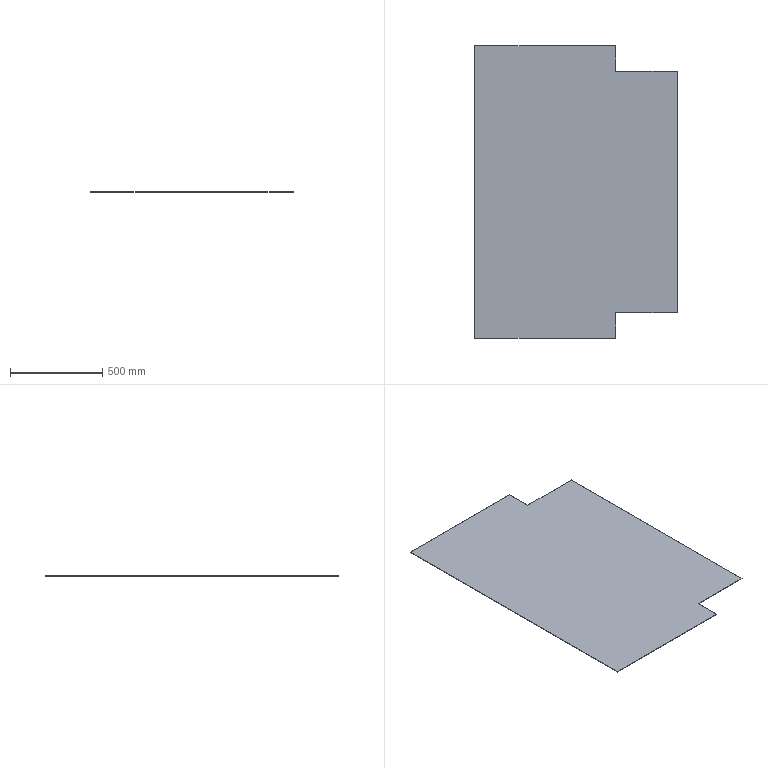Part | SolidWorks | 1 solid | 10 faces | box 1100 x 1590 x 2.5 mm | volume 4138000 mm3 | plane 10
STEP:
#1=CARTESIAN_POINT('',(-1620.,795.,0.));
#2=VERTEX_POINT('',#1);
#3=CARTESIAN_POINT('',(-1620.,-795.,0.));
#4=VERTEX_POINT('',#3);
#5=CARTESIAN_POINT('',(-1620.,795.,0.));
#6=DIRECTION('',(0.,-1.,0.));
#7=VECTOR('',#6,1000.);
#8=LINE('',#5,#7);
#9=EDGE_CURVE('',#2,#4,#8,.T.);
#10=ORIENTED_EDGE('',*,*,#9,.T.);
#11=CARTESIAN_POINT('',(-1620.,-795.,2.5));
#12=VERTEX_POINT('',#11);
#13=CARTESIAN_POINT('',(-1620.,-795.,2.5));
#14=DIRECTION('',(0.,0.,-1.));
#15=VECTOR('',#14,1000.);
#16=LINE('',#13,#15);
#17=EDGE_CURVE('',#12,#4,#16,.T.);
#18=ORIENTED_EDGE('',*,*,#17,.F.);
#19=CARTESIAN_POINT('',(-1620.,795.,2.5));
#20=VERTEX_POINT('',#19);
#21=CARTESIAN_POINT('',(-1620.,795.,2.5));
#22=DIRECTION('',(0.,-1.,0.));
#23=VECTOR('',#22,1000.);
#24=LINE('',#21,#23);
#25=EDGE_CURVE('',#20,#12,#24,.T.);
#26=ORIENTED_EDGE('',*,*,#25,.F.);
#27=CARTESIAN_POINT('',(-1620.,795.,2.5));
#28=DIRECTION('',(0.,0.,-1.));
#29=VECTOR('',#28,1000.);
#30=LINE('',#27,#29);
#31=EDGE_CURVE('',#20,#2,#30,.T.);
#32=ORIENTED_EDGE('',*,*,#31,.T.);
#33=EDGE_LOOP('',(#10,#18,#26,#32));
#34=FACE_OUTER_BOUND('',#33,.T.);
#35=CARTESIAN_POINT('',(-1620.,795.,2.5));
#36=DIRECTION('',(1.,0.,0.));
#37=DIRECTION('',(0.,1.,0.));
#38=AXIS2_PLACEMENT_3D('',#35,#36,#37);
#39=PLANE('',#38);
#40=ADVANCED_FACE('',(#34),#39,.F.);
#41=CARTESIAN_POINT('',(-855.,-795.,0.));
#42=VERTEX_POINT('',#41);
#43=CARTESIAN_POINT('',(-1620.,-795.,0.));
#44=DIRECTION('',(1.,0.,0.));
#45=VECTOR('',#44,1000.);
#46=LINE('',#43,#45);
#47=EDGE_CURVE('',#4,#42,#46,.T.);
#48=ORIENTED_EDGE('',*,*,#47,.T.);
#49=CARTESIAN_POINT('',(-855.,-795.,2.5));
#50=VERTEX_POINT('',#49);
#51=CARTESIAN_POINT('',(-855.,-795.,2.5));
#52=DIRECTION('',(0.,0.,-1.));
#53=VECTOR('',#52,1000.);
#54=LINE('',#51,#53);
#55=EDGE_CURVE('',#50,#42,#54,.T.);
#56=ORIENTED_EDGE('',*,*,#55,.F.);
#57=CARTESIAN_POINT('',(-1620.,-795.,2.5));
#58=DIRECTION('',(1.,0.,0.));
#59=VECTOR('',#58,1000.);
#60=LINE('',#57,#59);
#61=EDGE_CURVE('',#12,#50,#60,.T.);
#62=ORIENTED_EDGE('',*,*,#61,.F.);
#63=ORIENTED_EDGE('',*,*,#17,.T.);
#64=EDGE_LOOP('',(#48,#56,#62,#63));
#65=FACE_OUTER_BOUND('',#64,.T.);
#66=CARTESIAN_POINT('',(-1620.,-795.,2.5));
#67=DIRECTION('',(0.,1.,0.));
#68=DIRECTION('',(0.,0.,1.));
#69=AXIS2_PLACEMENT_3D('',#66,#67,#68);
#70=PLANE('',#69);
#71=ADVANCED_FACE('',(#65),#70,.F.);
#72=CARTESIAN_POINT('',(-855.,-655.,0.));
#73=VERTEX_POINT('',#72);
#74=CARTESIAN_POINT('',(-855.,-795.,0.));
#75=DIRECTION('',(0.,1.,0.));
#76=VECTOR('',#75,1000.);
#77=LINE('',#74,#76);
#78=EDGE_CURVE('',#42,#73,#77,.T.);
#79=ORIENTED_EDGE('',*,*,#78,.T.);
#80=CARTESIAN_POINT('',(-855.,-655.,2.5));
#81=VERTEX_POINT('',#80);
#82=CARTESIAN_POINT('',(-855.,-655.,2.5));
#83=DIRECTION('',(0.,0.,-1.));
#84=VECTOR('',#83,1000.);
#85=LINE('',#82,#84);
#86=EDGE_CURVE('',#81,#73,#85,.T.);
#87=ORIENTED_EDGE('',*,*,#86,.F.);
#88=CARTESIAN_POINT('',(-855.,-795.,2.5));
#89=DIRECTION('',(0.,1.,0.));
#90=VECTOR('',#89,1000.);
#91=LINE('',#88,#90);
#92=EDGE_CURVE('',#50,#81,#91,.T.);
#93=ORIENTED_EDGE('',*,*,#92,.F.);
#94=ORIENTED_EDGE('',*,*,#55,.T.);
#95=EDGE_LOOP('',(#79,#87,#93,#94));
#96=FACE_OUTER_BOUND('',#95,.T.);
#97=CARTESIAN_POINT('',(-855.,-795.,2.5));
#98=DIRECTION('',(-1.,0.,0.));
#99=DIRECTION('',(0.,0.,1.));
#100=AXIS2_PLACEMENT_3D('',#97,#98,#99);
#101=PLANE('',#100);
#102=ADVANCED_FACE('',(#96),#101,.F.);
#103=CARTESIAN_POINT('',(-520.,-655.,0.));
#104=VERTEX_POINT('',#103);
#105=CARTESIAN_POINT('',(-855.,-655.,0.));
#106=DIRECTION('',(1.,0.,0.));
#107=VECTOR('',#106,1000.);
#108=LINE('',#105,#107);
#109=EDGE_CURVE('',#73,#104,#108,.T.);
#110=ORIENTED_EDGE('',*,*,#109,.T.);
#111=CARTESIAN_POINT('',(-520.,-655.,2.5));
#112=VERTEX_POINT('',#111);
#113=CARTESIAN_POINT('',(-520.,-655.,2.5));
#114=DIRECTION('',(0.,0.,-1.));
#115=VECTOR('',#114,1000.);
#116=LINE('',#113,#115);
#117=EDGE_CURVE('',#112,#104,#116,.T.);
#118=ORIENTED_EDGE('',*,*,#117,.F.);
#119=CARTESIAN_POINT('',(-855.,-655.,2.5));
#120=DIRECTION('',(1.,0.,0.));
#121=VECTOR('',#120,1000.);
#122=LINE('',#119,#121);
#123=EDGE_CURVE('',#81,#112,#122,.T.);
#124=ORIENTED_EDGE('',*,*,#123,.F.);
#125=ORIENTED_EDGE('',*,*,#86,.T.);
#126=EDGE_LOOP('',(#110,#118,#124,#125));
#127=FACE_OUTER_BOUND('',#126,.T.);
#128=CARTESIAN_POINT('',(-855.,-655.,2.5));
#129=DIRECTION('',(0.,1.,0.));
#130=DIRECTION('',(0.,0.,1.));
#131=AXIS2_PLACEMENT_3D('',#128,#129,#130);
#132=PLANE('',#131);
#133=ADVANCED_FACE('',(#127),#132,.F.);
#134=CARTESIAN_POINT('',(-520.,655.,0.));
#135=VERTEX_POINT('',#134);
#136=CARTESIAN_POINT('',(-520.,655.,0.));
#137=DIRECTION('',(0.,1.,0.));
#138=VECTOR('',#137,1000.);
#139=LINE('',#136,#138);
#140=EDGE_CURVE('',#104,#135,#139,.T.);
#141=ORIENTED_EDGE('',*,*,#140,.T.);
#142=CARTESIAN_POINT('',(-520.,655.,2.5));
#143=VERTEX_POINT('',#142);
#144=CARTESIAN_POINT('',(-520.,655.,2.5));
#145=DIRECTION('',(0.,0.,-1.));
#146=VECTOR('',#145,1000.);
#147=LINE('',#144,#146);
#148=EDGE_CURVE('',#143,#135,#147,.T.);
#149=ORIENTED_EDGE('',*,*,#148,.F.);
#150=CARTESIAN_POINT('',(-520.,655.,2.5));
#151=DIRECTION('',(0.,1.,0.));
#152=VECTOR('',#151,1000.);
#153=LINE('',#150,#152);
#154=EDGE_CURVE('',#112,#143,#153,.T.);
#155=ORIENTED_EDGE('',*,*,#154,.F.);
#156=ORIENTED_EDGE('',*,*,#117,.T.);
#157=EDGE_LOOP('',(#141,#149,#155,#156));
#158=FACE_OUTER_BOUND('',#157,.T.);
#159=CARTESIAN_POINT('',(-520.,655.,2.5));
#160=DIRECTION('',(-1.,0.,0.));
#161=DIRECTION('',(0.,-1.,0.));
#162=AXIS2_PLACEMENT_3D('',#159,#160,#161);
#163=PLANE('',#162);
#164=ADVANCED_FACE('',(#158),#163,.F.);
#165=CARTESIAN_POINT('',(-855.,655.,0.));
#166=VERTEX_POINT('',#165);
#167=CARTESIAN_POINT('',(-855.,655.,0.));
#168=DIRECTION('',(-1.,0.,0.));
#169=VECTOR('',#168,1000.);
#170=LINE('',#167,#169);
#171=EDGE_CURVE('',#135,#166,#170,.T.);
#172=ORIENTED_EDGE('',*,*,#171,.T.);
#173=CARTESIAN_POINT('',(-855.,655.,2.5));
#174=VERTEX_POINT('',#173);
#175=CARTESIAN_POINT('',(-855.,655.,2.5));
#176=DIRECTION('',(0.,0.,-1.));
#177=VECTOR('',#176,1000.);
#178=LINE('',#175,#177);
#179=EDGE_CURVE('',#174,#166,#178,.T.);
#180=ORIENTED_EDGE('',*,*,#179,.F.);
#181=CARTESIAN_POINT('',(-855.,655.,2.5));
#182=DIRECTION('',(-1.,0.,0.));
#183=VECTOR('',#182,1000.);
#184=LINE('',#181,#183);
#185=EDGE_CURVE('',#143,#174,#184,.T.);
#186=ORIENTED_EDGE('',*,*,#185,.F.);
#187=ORIENTED_EDGE('',*,*,#148,.T.);
#188=EDGE_LOOP('',(#172,#180,#186,#187));
#189=FACE_OUTER_BOUND('',#188,.T.);
#190=CARTESIAN_POINT('',(-855.,655.,2.5));
#191=DIRECTION('',(0.,-1.,0.));
#192=DIRECTION('',(0.,0.,-1.));
#193=AXIS2_PLACEMENT_3D('',#190,#191,#192);
#194=PLANE('',#193);
#195=ADVANCED_FACE('',(#189),#194,.F.);
#196=CARTESIAN_POINT('',(-855.,795.,0.));
#197=VERTEX_POINT('',#196);
#198=CARTESIAN_POINT('',(-855.,795.,0.));
#199=DIRECTION('',(0.,1.,0.));
#200=VECTOR('',#199,1000.);
#201=LINE('',#198,#200);
#202=EDGE_CURVE('',#166,#197,#201,.T.);
#203=ORIENTED_EDGE('',*,*,#202,.T.);
#204=CARTESIAN_POINT('',(-855.,795.,2.5));
#205=VERTEX_POINT('',#204);
#206=CARTESIAN_POINT('',(-855.,795.,2.5));
#207=DIRECTION('',(0.,0.,-1.));
#208=VECTOR('',#207,1000.);
#209=LINE('',#206,#208);
#210=EDGE_CURVE('',#205,#197,#209,.T.);
#211=ORIENTED_EDGE('',*,*,#210,.F.);
#212=CARTESIAN_POINT('',(-855.,795.,2.5));
#213=DIRECTION('',(0.,1.,0.));
#214=VECTOR('',#213,1000.);
#215=LINE('',#212,#214);
#216=EDGE_CURVE('',#174,#205,#215,.T.);
#217=ORIENTED_EDGE('',*,*,#216,.F.);
#218=ORIENTED_EDGE('',*,*,#179,.T.);
#219=EDGE_LOOP('',(#203,#211,#217,#218));
#220=FACE_OUTER_BOUND('',#219,.T.);
#221=CARTESIAN_POINT('',(-855.,795.,2.5));
#222=DIRECTION('',(-1.,0.,0.));
#223=DIRECTION('',(0.,0.,1.));
#224=AXIS2_PLACEMENT_3D('',#221,#222,#223);
#225=PLANE('',#224);
#226=ADVANCED_FACE('',(#220),#225,.F.);
#227=CARTESIAN_POINT('',(-1620.,795.,0.));
#228=DIRECTION('',(-1.,0.,0.));
#229=VECTOR('',#228,1000.);
#230=LINE('',#227,#229);
#231=EDGE_CURVE('',#197,#2,#230,.T.);
#232=ORIENTED_EDGE('',*,*,#231,.T.);
#233=ORIENTED_EDGE('',*,*,#31,.F.);
#234=CARTESIAN_POINT('',(-1620.,795.,2.5));
#235=DIRECTION('',(-1.,0.,0.));
#236=VECTOR('',#235,1000.);
#237=LINE('',#234,#236);
#238=EDGE_CURVE('',#205,#20,#237,.T.);
#239=ORIENTED_EDGE('',*,*,#238,.F.);
#240=ORIENTED_EDGE('',*,*,#210,.T.);
#241=EDGE_LOOP('',(#232,#233,#239,#240));
#242=FACE_OUTER_BOUND('',#241,.T.);
#243=CARTESIAN_POINT('',(-1620.,795.,2.5));
#244=DIRECTION('',(0.,-1.,0.));
#245=DIRECTION('',(0.,0.,-1.));
#246=AXIS2_PLACEMENT_3D('',#243,#244,#245);
#247=PLANE('',#246);
#248=ADVANCED_FACE('',(#242),#247,.F.);
#249=ORIENTED_EDGE('',*,*,#25,.T.);
#250=ORIENTED_EDGE('',*,*,#61,.T.);
#251=ORIENTED_EDGE('',*,*,#92,.T.);
#252=ORIENTED_EDGE('',*,*,#123,.T.);
#253=ORIENTED_EDGE('',*,*,#154,.T.);
#254=ORIENTED_EDGE('',*,*,#185,.T.);
#255=ORIENTED_EDGE('',*,*,#216,.T.);
#256=ORIENTED_EDGE('',*,*,#238,.T.);
#257=EDGE_LOOP('',(#249,#250,#251,#252,#253,#254,#255,#256));
#258=FACE_OUTER_BOUND('',#257,.T.);
#259=CARTESIAN_POINT('',(0.,0.,2.5));
#260=DIRECTION('',(0.,0.,1.));
#261=DIRECTION('',(1.,0.,0.));
#262=AXIS2_PLACEMENT_3D('',#259,#260,#261);
#263=PLANE('',#262);
#264=ADVANCED_FACE('',(#258),#263,.T.);
#265=ORIENTED_EDGE('',*,*,#9,.F.);
#266=ORIENTED_EDGE('',*,*,#231,.F.);
#267=ORIENTED_EDGE('',*,*,#202,.F.);
#268=ORIENTED_EDGE('',*,*,#171,.F.);
#269=ORIENTED_EDGE('',*,*,#140,.F.);
#270=ORIENTED_EDGE('',*,*,#109,.F.);
#271=ORIENTED_EDGE('',*,*,#78,.F.);
#272=ORIENTED_EDGE('',*,*,#47,.F.);
#273=EDGE_LOOP('',(#265,#266,#267,#268,#269,#270,#271,#272));
#274=FACE_OUTER_BOUND('',#273,.T.);
#275=CARTESIAN_POINT('',(0.,0.,0.));
#276=DIRECTION('',(0.,0.,1.));
#277=DIRECTION('',(1.,0.,0.));
#278=AXIS2_PLACEMENT_3D('',#275,#276,#277);
#279=PLANE('',#278);
#280=ADVANCED_FACE('',(#274),#279,.F.);
#281=CLOSED_SHELL('',(#40,#71,#102,#133,#164,#195,#226,#248,#264,#280));
#282=MANIFOLD_SOLID_BREP('',#281);
#283=CARTESIAN_POINT('',(0.,0.,0.));
#284=DIRECTION('',(0.,0.,1.));
#285=DIRECTION('',(1.,0.,0.));
#286=AXIS2_PLACEMENT_3D('',#283,#284,#285);
#287=(LENGTH_UNIT()NAMED_UNIT(*)SI_UNIT(.MILLI.,.METRE.));
#288=UNCERTAINTY_MEASURE_WITH_UNIT(LENGTH_MEASURE(0.00001),#287,'','');
#289=(NAMED_UNIT(*)PLANE_ANGLE_UNIT()SI_UNIT($,.RADIAN.));
#290=(NAMED_UNIT(*)SI_UNIT($,.STERADIAN.)SOLID_ANGLE_UNIT());
#291=(GEOMETRIC_REPRESENTATION_CONTEXT(3)GLOBAL_UNCERTAINTY_ASSIGNED_CONTEXT((#288))GLOBAL_UNIT_ASSIGNED_CONTEXT((#287,#289,#290))REPRESENTATION_CONTEXT('',''));
#292=ADVANCED_BREP_SHAPE_REPRESENTATION('',(#282,#286),#291);